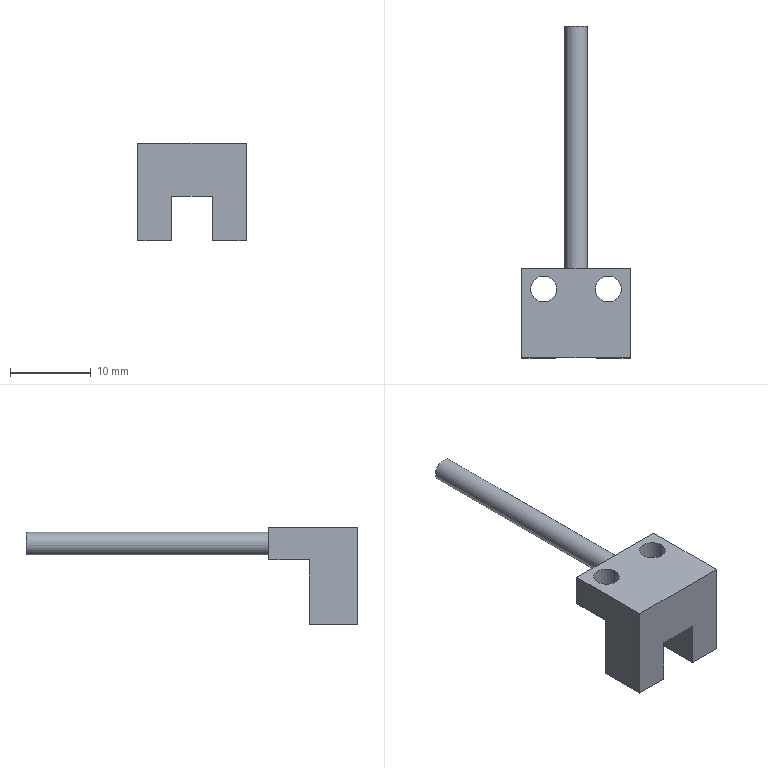Part | STEP file | 1 solid | 16 faces | box 13.4 x 41 x 12 mm | volume 1188 mm3 | plane 13 | cylinder 3 | commonest cylinder face diameters 3.2 x2 2.8 x1
STEP:
#1=CARTESIAN_POINT('',(0.,0.,0.));
#2=DIRECTION('',(0.,0.,1.));
#3=DIRECTION('',(1.,0.,0.));
#4=AXIS2_PLACEMENT_3D('',#1,#2,#3);
#5=CARTESIAN_POINT('',(2.5,0.,-0.5));
#6=VERTEX_POINT('',#5);
#7=CARTESIAN_POINT('',(2.5,0.,-6.));
#8=VERTEX_POINT('',#7);
#9=CARTESIAN_POINT('',(2.5,0.,0.));
#10=DIRECTION('',(0.,0.,-1.));
#11=VECTOR('',#10,1.);
#12=LINE('',#9,#11);
#13=CARTESIAN_POINT('',(0.,0.,0.));
#14=DIRECTION('',(0.,-1.,0.));
#15=DIRECTION('',(0.,0.,-1.));
#16=AXIS2_PLACEMENT_3D('',#13,#14,#15);
#17=PLANE('',#16);
#18=CARTESIAN_POINT('',(0.,2.5));
#19=DIRECTION('',(1.,0.));
#20=VECTOR('',#19,1.);
#21=LINE('',#18,#20);
#22=(GEOMETRIC_REPRESENTATION_CONTEXT(2)PARAMETRIC_REPRESENTATION_CONTEXT()REPRESENTATION_CONTEXT('',''));
#23=DEFINITIONAL_REPRESENTATION('',(#21),#22);
#24=PCURVE('',#17,#23);
#25=CARTESIAN_POINT('',(2.5,11.,-6.));
#26=DIRECTION('',(1.,0.,0.));
#27=DIRECTION('',(0.,0.,-1.));
#28=AXIS2_PLACEMENT_3D('',#25,#26,#27);
#29=PLANE('',#28);
#30=CARTESIAN_POINT('',(-6.,-11.));
#31=DIRECTION('',(1.,0.));
#32=VECTOR('',#31,1.);
#33=LINE('',#30,#32);
#34=(GEOMETRIC_REPRESENTATION_CONTEXT(2)PARAMETRIC_REPRESENTATION_CONTEXT()REPRESENTATION_CONTEXT('',''));
#35=DEFINITIONAL_REPRESENTATION('',(#33),#34);
#36=PCURVE('',#29,#35);
#37=SURFACE_CURVE('',#12,(#24,#36),.PCURVE_S1.);
#38=EDGE_CURVE('',#6,#8,#37,.T.);
#39=ORIENTED_EDGE('',*,*,#38,.T.);
#40=CARTESIAN_POINT('',(6.7,0.,-6.));
#41=VERTEX_POINT('',#40);
#42=CARTESIAN_POINT('',(0.,0.,-6.));
#43=DIRECTION('',(1.,0.,0.));
#44=VECTOR('',#43,1.);
#45=LINE('',#42,#44);
#46=CARTESIAN_POINT('',(6.,0.));
#47=DIRECTION('',(0.,1.));
#48=VECTOR('',#47,1.);
#49=LINE('',#46,#48);
#50=(GEOMETRIC_REPRESENTATION_CONTEXT(2)PARAMETRIC_REPRESENTATION_CONTEXT()REPRESENTATION_CONTEXT('',''));
#51=DEFINITIONAL_REPRESENTATION('',(#49),#50);
#52=PCURVE('',#17,#51);
#53=CARTESIAN_POINT('',(2.5,11.,-6.));
#54=DIRECTION('',(0.,0.,1.));
#55=DIRECTION('',(1.,0.,0.));
#56=AXIS2_PLACEMENT_3D('',#53,#54,#55);
#57=PLANE('',#56);
#58=CARTESIAN_POINT('',(-2.5,-11.));
#59=DIRECTION('',(1.,0.));
#60=VECTOR('',#59,1.);
#61=LINE('',#58,#60);
#62=(GEOMETRIC_REPRESENTATION_CONTEXT(2)PARAMETRIC_REPRESENTATION_CONTEXT()REPRESENTATION_CONTEXT('',''));
#63=DEFINITIONAL_REPRESENTATION('',(#61),#62);
#64=PCURVE('',#57,#63);
#65=SURFACE_CURVE('',#45,(#52,#64),.PCURVE_S1.);
#66=EDGE_CURVE('',#8,#41,#65,.T.);
#67=ORIENTED_EDGE('',*,*,#66,.T.);
#68=CARTESIAN_POINT('',(6.7,0.,6.));
#69=VERTEX_POINT('',#68);
#70=CARTESIAN_POINT('',(6.7,0.,0.));
#71=DIRECTION('',(0.,0.,1.));
#72=VECTOR('',#71,1.);
#73=LINE('',#70,#72);
#74=CARTESIAN_POINT('',(0.,6.7));
#75=DIRECTION('',(-1.,0.));
#76=VECTOR('',#75,1.);
#77=LINE('',#74,#76);
#78=(GEOMETRIC_REPRESENTATION_CONTEXT(2)PARAMETRIC_REPRESENTATION_CONTEXT()REPRESENTATION_CONTEXT('',''));
#79=DEFINITIONAL_REPRESENTATION('',(#77),#78);
#80=PCURVE('',#17,#79);
#81=CARTESIAN_POINT('',(6.7,11.,6.));
#82=DIRECTION('',(-1.,0.,0.));
#83=DIRECTION('',(0.,0.,1.));
#84=AXIS2_PLACEMENT_3D('',#81,#82,#83);
#85=PLANE('',#84);
#86=CARTESIAN_POINT('',(-6.,-11.));
#87=DIRECTION('',(1.,0.));
#88=VECTOR('',#87,1.);
#89=LINE('',#86,#88);
#90=(GEOMETRIC_REPRESENTATION_CONTEXT(2)PARAMETRIC_REPRESENTATION_CONTEXT()REPRESENTATION_CONTEXT('',''));
#91=DEFINITIONAL_REPRESENTATION('',(#89),#90);
#92=PCURVE('',#85,#91);
#93=SURFACE_CURVE('',#73,(#80,#92),.PCURVE_S1.);
#94=EDGE_CURVE('',#41,#69,#93,.T.);
#95=ORIENTED_EDGE('',*,*,#94,.T.);
#96=CARTESIAN_POINT('',(-6.7,0.,6.));
#97=VERTEX_POINT('',#96);
#98=CARTESIAN_POINT('',(0.,0.,6.));
#99=DIRECTION('',(-1.,0.,0.));
#100=VECTOR('',#99,1.);
#101=LINE('',#98,#100);
#102=CARTESIAN_POINT('',(-6.,0.));
#103=DIRECTION('',(0.,-1.));
#104=VECTOR('',#103,1.);
#105=LINE('',#102,#104);
#106=(GEOMETRIC_REPRESENTATION_CONTEXT(2)PARAMETRIC_REPRESENTATION_CONTEXT()REPRESENTATION_CONTEXT('',''));
#107=DEFINITIONAL_REPRESENTATION('',(#105),#106);
#108=PCURVE('',#17,#107);
#109=CARTESIAN_POINT('',(-6.7,11.,6.));
#110=DIRECTION('',(0.,0.,-1.));
#111=DIRECTION('',(-1.,0.,0.));
#112=AXIS2_PLACEMENT_3D('',#109,#110,#111);
#113=PLANE('',#112);
#114=CARTESIAN_POINT('',(-6.7,-11.));
#115=DIRECTION('',(1.,0.));
#116=VECTOR('',#115,1.);
#117=LINE('',#114,#116);
#118=(GEOMETRIC_REPRESENTATION_CONTEXT(2)PARAMETRIC_REPRESENTATION_CONTEXT()REPRESENTATION_CONTEXT('',''));
#119=DEFINITIONAL_REPRESENTATION('',(#117),#118);
#120=PCURVE('',#113,#119);
#121=SURFACE_CURVE('',#101,(#108,#120),.PCURVE_S1.);
#122=EDGE_CURVE('',#69,#97,#121,.T.);
#123=ORIENTED_EDGE('',*,*,#122,.T.);
#124=CARTESIAN_POINT('',(-6.7,0.,-6.));
#125=VERTEX_POINT('',#124);
#126=CARTESIAN_POINT('',(-6.7,0.,0.));
#127=DIRECTION('',(0.,0.,-1.));
#128=VECTOR('',#127,1.);
#129=LINE('',#126,#128);
#130=CARTESIAN_POINT('',(0.,-6.7));
#131=DIRECTION('',(1.,0.));
#132=VECTOR('',#131,1.);
#133=LINE('',#130,#132);
#134=(GEOMETRIC_REPRESENTATION_CONTEXT(2)PARAMETRIC_REPRESENTATION_CONTEXT()REPRESENTATION_CONTEXT('',''));
#135=DEFINITIONAL_REPRESENTATION('',(#133),#134);
#136=PCURVE('',#17,#135);
#137=CARTESIAN_POINT('',(-6.7,11.,6.));
#138=DIRECTION('',(1.,0.,0.));
#139=DIRECTION('',(0.,0.,-1.));
#140=AXIS2_PLACEMENT_3D('',#137,#138,#139);
#141=PLANE('',#140);
#142=CARTESIAN_POINT('',(6.,-11.));
#143=DIRECTION('',(1.,0.));
#144=VECTOR('',#143,1.);
#145=LINE('',#142,#144);
#146=(GEOMETRIC_REPRESENTATION_CONTEXT(2)PARAMETRIC_REPRESENTATION_CONTEXT()REPRESENTATION_CONTEXT('',''));
#147=DEFINITIONAL_REPRESENTATION('',(#145),#146);
#148=PCURVE('',#141,#147);
#149=SURFACE_CURVE('',#129,(#136,#148),.PCURVE_S1.);
#150=EDGE_CURVE('',#97,#125,#149,.T.);
#151=ORIENTED_EDGE('',*,*,#150,.T.);
#152=CARTESIAN_POINT('',(-2.5,0.,-6.));
#153=VERTEX_POINT('',#152);
#154=CARTESIAN_POINT('',(0.,0.,-6.));
#155=DIRECTION('',(1.,0.,0.));
#156=VECTOR('',#155,1.);
#157=LINE('',#154,#156);
#158=CARTESIAN_POINT('',(6.,0.));
#159=DIRECTION('',(0.,1.));
#160=VECTOR('',#159,1.);
#161=LINE('',#158,#160);
#162=(GEOMETRIC_REPRESENTATION_CONTEXT(2)PARAMETRIC_REPRESENTATION_CONTEXT()REPRESENTATION_CONTEXT('',''));
#163=DEFINITIONAL_REPRESENTATION('',(#161),#162);
#164=PCURVE('',#17,#163);
#165=CARTESIAN_POINT('',(-6.7,11.,-6.));
#166=DIRECTION('',(0.,0.,1.));
#167=DIRECTION('',(1.,0.,0.));
#168=AXIS2_PLACEMENT_3D('',#165,#166,#167);
#169=PLANE('',#168);
#170=CARTESIAN_POINT('',(6.7,-11.));
#171=DIRECTION('',(1.,0.));
#172=VECTOR('',#171,1.);
#173=LINE('',#170,#172);
#174=(GEOMETRIC_REPRESENTATION_CONTEXT(2)PARAMETRIC_REPRESENTATION_CONTEXT()REPRESENTATION_CONTEXT('',''));
#175=DEFINITIONAL_REPRESENTATION('',(#173),#174);
#176=PCURVE('',#169,#175);
#177=SURFACE_CURVE('',#157,(#164,#176),.PCURVE_S1.);
#178=EDGE_CURVE('',#125,#153,#177,.T.);
#179=ORIENTED_EDGE('',*,*,#178,.T.);
#180=CARTESIAN_POINT('',(-2.5,0.,-0.5));
#181=VERTEX_POINT('',#180);
#182=CARTESIAN_POINT('',(-2.5,0.,0.));
#183=DIRECTION('',(0.,0.,1.));
#184=VECTOR('',#183,1.);
#185=LINE('',#182,#184);
#186=CARTESIAN_POINT('',(0.,-2.5));
#187=DIRECTION('',(-1.,0.));
#188=VECTOR('',#187,1.);
#189=LINE('',#186,#188);
#190=(GEOMETRIC_REPRESENTATION_CONTEXT(2)PARAMETRIC_REPRESENTATION_CONTEXT()REPRESENTATION_CONTEXT('',''));
#191=DEFINITIONAL_REPRESENTATION('',(#189),#190);
#192=PCURVE('',#17,#191);
#193=CARTESIAN_POINT('',(-2.5,11.,-6.));
#194=DIRECTION('',(-1.,0.,0.));
#195=DIRECTION('',(0.,0.,1.));
#196=AXIS2_PLACEMENT_3D('',#193,#194,#195);
#197=PLANE('',#196);
#198=CARTESIAN_POINT('',(6.,-11.));
#199=DIRECTION('',(1.,0.));
#200=VECTOR('',#199,1.);
#201=LINE('',#198,#200);
#202=(GEOMETRIC_REPRESENTATION_CONTEXT(2)PARAMETRIC_REPRESENTATION_CONTEXT()REPRESENTATION_CONTEXT('',''));
#203=DEFINITIONAL_REPRESENTATION('',(#201),#202);
#204=PCURVE('',#197,#203);
#205=SURFACE_CURVE('',#185,(#192,#204),.PCURVE_S1.);
#206=EDGE_CURVE('',#153,#181,#205,.T.);
#207=ORIENTED_EDGE('',*,*,#206,.T.);
#208=CARTESIAN_POINT('',(0.,0.,-0.5));
#209=DIRECTION('',(1.,0.,0.));
#210=VECTOR('',#209,1.);
#211=LINE('',#208,#210);
#212=CARTESIAN_POINT('',(0.5,0.));
#213=DIRECTION('',(0.,1.));
#214=VECTOR('',#213,1.);
#215=LINE('',#212,#214);
#216=(GEOMETRIC_REPRESENTATION_CONTEXT(2)PARAMETRIC_REPRESENTATION_CONTEXT()REPRESENTATION_CONTEXT('',''));
#217=DEFINITIONAL_REPRESENTATION('',(#215),#216);
#218=PCURVE('',#17,#217);
#219=CARTESIAN_POINT('',(-2.5,11.,-0.5));
#220=DIRECTION('',(0.,0.,1.));
#221=DIRECTION('',(0.,-1.,0.));
#222=AXIS2_PLACEMENT_3D('',#219,#220,#221);
#223=PLANE('',#222);
#224=CARTESIAN_POINT('',(11.,2.5));
#225=DIRECTION('',(0.,1.));
#226=VECTOR('',#225,1.);
#227=LINE('',#224,#226);
#228=(GEOMETRIC_REPRESENTATION_CONTEXT(2)PARAMETRIC_REPRESENTATION_CONTEXT()REPRESENTATION_CONTEXT('',''));
#229=DEFINITIONAL_REPRESENTATION('',(#227),#228);
#230=PCURVE('',#223,#229);
#231=SURFACE_CURVE('',#211,(#218,#230),.PCURVE_S1.);
#232=EDGE_CURVE('',#181,#6,#231,.T.);
#233=ORIENTED_EDGE('',*,*,#232,.T.);
#234=EDGE_LOOP('',(#39,#67,#95,#123,#151,#179,#207,#233));
#235=FACE_BOUND('',#234,.T.);
#236=ADVANCED_FACE('',(#235),#17,.T.);
#237=CARTESIAN_POINT('',(6.7,6.,-6.));
#238=VERTEX_POINT('',#237);
#239=CARTESIAN_POINT('',(6.7,11.,-6.));
#240=DIRECTION('',(0.,1.,0.));
#241=VECTOR('',#240,1.);
#242=LINE('',#239,#241);
#243=CARTESIAN_POINT('',(4.2,0.));
#244=DIRECTION('',(0.,1.));
#245=VECTOR('',#244,1.);
#246=LINE('',#243,#245);
#247=(GEOMETRIC_REPRESENTATION_CONTEXT(2)PARAMETRIC_REPRESENTATION_CONTEXT()REPRESENTATION_CONTEXT('',''));
#248=DEFINITIONAL_REPRESENTATION('',(#246),#247);
#249=PCURVE('',#57,#248);
#250=CARTESIAN_POINT('',(-12.,0.));
#251=DIRECTION('',(0.,1.));
#252=VECTOR('',#251,1.);
#253=LINE('',#250,#252);
#254=(GEOMETRIC_REPRESENTATION_CONTEXT(2)PARAMETRIC_REPRESENTATION_CONTEXT()REPRESENTATION_CONTEXT('',''));
#255=DEFINITIONAL_REPRESENTATION('',(#253),#254);
#256=PCURVE('',#85,#255);
#257=SURFACE_CURVE('',#242,(#249,#256),.PCURVE_S1.);
#258=EDGE_CURVE('',#41,#238,#257,.T.);
#259=ORIENTED_EDGE('',*,*,#258,.F.);
#260=ORIENTED_EDGE('',*,*,#66,.F.);
#261=CARTESIAN_POINT('',(2.5,6.,-6.));
#262=VERTEX_POINT('',#261);
#263=CARTESIAN_POINT('',(2.5,11.,-6.));
#264=DIRECTION('',(0.,-1.,0.));
#265=VECTOR('',#264,1.);
#266=LINE('',#263,#265);
#267=CARTESIAN_POINT('',(0.,0.));
#268=DIRECTION('',(0.,-1.));
#269=VECTOR('',#268,1.);
#270=LINE('',#267,#269);
#271=(GEOMETRIC_REPRESENTATION_CONTEXT(2)PARAMETRIC_REPRESENTATION_CONTEXT()REPRESENTATION_CONTEXT('',''));
#272=DEFINITIONAL_REPRESENTATION('',(#270),#271);
#273=PCURVE('',#57,#272);
#274=CARTESIAN_POINT('',(0.,0.));
#275=DIRECTION('',(0.,-1.));
#276=VECTOR('',#275,1.);
#277=LINE('',#274,#276);
#278=(GEOMETRIC_REPRESENTATION_CONTEXT(2)PARAMETRIC_REPRESENTATION_CONTEXT()REPRESENTATION_CONTEXT('',''));
#279=DEFINITIONAL_REPRESENTATION('',(#277),#278);
#280=PCURVE('',#29,#279);
#281=SURFACE_CURVE('',#266,(#273,#280),.PCURVE_S1.);
#282=EDGE_CURVE('',#262,#8,#281,.T.);
#283=ORIENTED_EDGE('',*,*,#282,.F.);
#284=CARTESIAN_POINT('',(2.5,6.,-6.));
#285=DIRECTION('',(-1.,0.,0.));
#286=VECTOR('',#285,1.);
#287=LINE('',#284,#286);
#288=CARTESIAN_POINT('',(0.,-5.));
#289=DIRECTION('',(-1.,0.));
#290=VECTOR('',#289,1.);
#291=LINE('',#288,#290);
#292=(GEOMETRIC_REPRESENTATION_CONTEXT(2)PARAMETRIC_REPRESENTATION_CONTEXT()REPRESENTATION_CONTEXT('',''));
#293=DEFINITIONAL_REPRESENTATION('',(#291),#292);
#294=PCURVE('',#57,#293);
#295=CARTESIAN_POINT('',(0.,6.,0.));
#296=DIRECTION('',(0.,1.,0.));
#297=DIRECTION('',(0.,0.,1.));
#298=AXIS2_PLACEMENT_3D('',#295,#296,#297);
#299=PLANE('',#298);
#300=CARTESIAN_POINT('',(-6.,2.5));
#301=DIRECTION('',(0.,-1.));
#302=VECTOR('',#301,1.);
#303=LINE('',#300,#302);
#304=(GEOMETRIC_REPRESENTATION_CONTEXT(2)PARAMETRIC_REPRESENTATION_CONTEXT()REPRESENTATION_CONTEXT('',''));
#305=DEFINITIONAL_REPRESENTATION('',(#303),#304);
#306=PCURVE('',#299,#305);
#307=SURFACE_CURVE('',#287,(#294,#306),.PCURVE_S1.);
#308=EDGE_CURVE('',#238,#262,#307,.T.);
#309=ORIENTED_EDGE('',*,*,#308,.F.);
#310=EDGE_LOOP('',(#259,#260,#283,#309));
#311=FACE_BOUND('',#310,.T.);
#312=ADVANCED_FACE('',(#311),#57,.F.);
#313=ORIENTED_EDGE('',*,*,#282,.T.);
#314=ORIENTED_EDGE('',*,*,#38,.F.);
#315=CARTESIAN_POINT('',(2.5,6.,-0.5));
#316=VERTEX_POINT('',#315);
#317=CARTESIAN_POINT('',(2.5,11.,-0.5));
#318=DIRECTION('',(0.,-1.,0.));
#319=VECTOR('',#318,1.);
#320=LINE('',#317,#319);
#321=CARTESIAN_POINT('',(-5.5,0.));
#322=DIRECTION('',(0.,-1.));
#323=VECTOR('',#322,1.);
#324=LINE('',#321,#323);
#325=(GEOMETRIC_REPRESENTATION_CONTEXT(2)PARAMETRIC_REPRESENTATION_CONTEXT()REPRESENTATION_CONTEXT('',''));
#326=DEFINITIONAL_REPRESENTATION('',(#324),#325);
#327=PCURVE('',#29,#326);
#328=CARTESIAN_POINT('',(0.,5.));
#329=DIRECTION('',(1.,0.));
#330=VECTOR('',#329,1.);
#331=LINE('',#328,#330);
#332=(GEOMETRIC_REPRESENTATION_CONTEXT(2)PARAMETRIC_REPRESENTATION_CONTEXT()REPRESENTATION_CONTEXT('',''));
#333=DEFINITIONAL_REPRESENTATION('',(#331),#332);
#334=PCURVE('',#223,#333);
#335=SURFACE_CURVE('',#320,(#327,#334),.PCURVE_S1.);
#336=EDGE_CURVE('',#316,#6,#335,.T.);
#337=ORIENTED_EDGE('',*,*,#336,.F.);
#338=CARTESIAN_POINT('',(2.5,6.,-6.));
#339=DIRECTION('',(0.,0.,1.));
#340=VECTOR('',#339,1.);
#341=LINE('',#338,#340);
#342=CARTESIAN_POINT('',(0.,-5.));
#343=DIRECTION('',(-1.,0.));
#344=VECTOR('',#343,1.);
#345=LINE('',#342,#344);
#346=(GEOMETRIC_REPRESENTATION_CONTEXT(2)PARAMETRIC_REPRESENTATION_CONTEXT()REPRESENTATION_CONTEXT('',''));
#347=DEFINITIONAL_REPRESENTATION('',(#345),#346);
#348=PCURVE('',#29,#347);
#349=CARTESIAN_POINT('',(-6.,2.5));
#350=DIRECTION('',(1.,0.));
#351=VECTOR('',#350,1.);
#352=LINE('',#349,#351);
#353=(GEOMETRIC_REPRESENTATION_CONTEXT(2)PARAMETRIC_REPRESENTATION_CONTEXT()REPRESENTATION_CONTEXT('',''));
#354=DEFINITIONAL_REPRESENTATION('',(#352),#353);
#355=PCURVE('',#299,#354);
#356=SURFACE_CURVE('',#341,(#348,#355),.PCURVE_S1.);
#357=EDGE_CURVE('',#262,#316,#356,.T.);
#358=ORIENTED_EDGE('',*,*,#357,.F.);
#359=EDGE_LOOP('',(#313,#314,#337,#358));
#360=FACE_BOUND('',#359,.T.);
#361=ADVANCED_FACE('',(#360),#29,.F.);
#362=ORIENTED_EDGE('',*,*,#336,.T.);
#363=ORIENTED_EDGE('',*,*,#232,.F.);
#364=CARTESIAN_POINT('',(-2.5,6.,-0.5));
#365=VERTEX_POINT('',#364);
#366=CARTESIAN_POINT('',(-2.5,11.,-0.5));
#367=DIRECTION('',(0.,-1.,0.));
#368=VECTOR('',#367,1.);
#369=LINE('',#366,#368);
#370=CARTESIAN_POINT('',(0.,0.));
#371=DIRECTION('',(1.,0.));
#372=VECTOR('',#371,1.);
#373=LINE('',#370,#372);
#374=(GEOMETRIC_REPRESENTATION_CONTEXT(2)PARAMETRIC_REPRESENTATION_CONTEXT()REPRESENTATION_CONTEXT('',''));
#375=DEFINITIONAL_REPRESENTATION('',(#373),#374);
#376=PCURVE('',#223,#375);
#377=CARTESIAN_POINT('',(5.5,0.));
#378=DIRECTION('',(0.,-1.));
#379=VECTOR('',#378,1.);
#380=LINE('',#377,#379);
#381=(GEOMETRIC_REPRESENTATION_CONTEXT(2)PARAMETRIC_REPRESENTATION_CONTEXT()REPRESENTATION_CONTEXT('',''));
#382=DEFINITIONAL_REPRESENTATION('',(#380),#381);
#383=PCURVE('',#197,#382);
#384=SURFACE_CURVE('',#369,(#376,#383),.PCURVE_S1.);
#385=EDGE_CURVE('',#365,#181,#384,.T.);
#386=ORIENTED_EDGE('',*,*,#385,.F.);
#387=CARTESIAN_POINT('',(-2.5,6.,-0.5));
#388=DIRECTION('',(-1.,0.,0.));
#389=VECTOR('',#388,1.);
#390=LINE('',#387,#389);
#391=CARTESIAN_POINT('',(5.,0.));
#392=DIRECTION('',(0.,-1.));
#393=VECTOR('',#392,1.);
#394=LINE('',#391,#393);
#395=(GEOMETRIC_REPRESENTATION_CONTEXT(2)PARAMETRIC_REPRESENTATION_CONTEXT()REPRESENTATION_CONTEXT('',''));
#396=DEFINITIONAL_REPRESENTATION('',(#394),#395);
#397=PCURVE('',#223,#396);
#398=CARTESIAN_POINT('',(-0.5,-2.5));
#399=DIRECTION('',(0.,-1.));
#400=VECTOR('',#399,1.);
#401=LINE('',#398,#400);
#402=(GEOMETRIC_REPRESENTATION_CONTEXT(2)PARAMETRIC_REPRESENTATION_CONTEXT()REPRESENTATION_CONTEXT('',''));
#403=DEFINITIONAL_REPRESENTATION('',(#401),#402);
#404=PCURVE('',#299,#403);
#405=SURFACE_CURVE('',#390,(#397,#404),.PCURVE_S1.);
#406=EDGE_CURVE('',#316,#365,#405,.T.);
#407=ORIENTED_EDGE('',*,*,#406,.F.);
#408=EDGE_LOOP('',(#362,#363,#386,#407));
#409=FACE_BOUND('',#408,.T.);
#410=ADVANCED_FACE('',(#409),#223,.F.);
#411=ORIENTED_EDGE('',*,*,#385,.T.);
#412=ORIENTED_EDGE('',*,*,#206,.F.);
#413=CARTESIAN_POINT('',(-2.5,6.,-6.));
#414=VERTEX_POINT('',#413);
#415=CARTESIAN_POINT('',(-2.5,11.,-6.));
#416=DIRECTION('',(0.,-1.,0.));
#417=VECTOR('',#416,1.);
#418=LINE('',#415,#417);
#419=CARTESIAN_POINT('',(0.,0.));
#420=DIRECTION('',(0.,-1.));
#421=VECTOR('',#420,1.);
#422=LINE('',#419,#421);
#423=(GEOMETRIC_REPRESENTATION_CONTEXT(2)PARAMETRIC_REPRESENTATION_CONTEXT()REPRESENTATION_CONTEXT('',''));
#424=DEFINITIONAL_REPRESENTATION('',(#422),#423);
#425=PCURVE('',#197,#424);
#426=CARTESIAN_POINT('',(4.2,0.));
#427=DIRECTION('',(0.,-1.));
#428=VECTOR('',#427,1.);
#429=LINE('',#426,#428);
#430=(GEOMETRIC_REPRESENTATION_CONTEXT(2)PARAMETRIC_REPRESENTATION_CONTEXT()REPRESENTATION_CONTEXT('',''));
#431=DEFINITIONAL_REPRESENTATION('',(#429),#430);
#432=PCURVE('',#169,#431);
#433=SURFACE_CURVE('',#418,(#425,#432),.PCURVE_S1.);
#434=EDGE_CURVE('',#414,#153,#433,.T.);
#435=ORIENTED_EDGE('',*,*,#434,.F.);
#436=CARTESIAN_POINT('',(-2.5,6.,-6.));
#437=DIRECTION('',(0.,0.,-1.));
#438=VECTOR('',#437,1.);
#439=LINE('',#436,#438);
#440=CARTESIAN_POINT('',(0.,-5.));
#441=DIRECTION('',(-1.,0.));
#442=VECTOR('',#441,1.);
#443=LINE('',#440,#442);
#444=(GEOMETRIC_REPRESENTATION_CONTEXT(2)PARAMETRIC_REPRESENTATION_CONTEXT()REPRESENTATION_CONTEXT('',''));
#445=DEFINITIONAL_REPRESENTATION('',(#443),#444);
#446=PCURVE('',#197,#445);
#447=CARTESIAN_POINT('',(-6.,-2.5));
#448=DIRECTION('',(-1.,0.));
#449=VECTOR('',#448,1.);
#450=LINE('',#447,#449);
#451=(GEOMETRIC_REPRESENTATION_CONTEXT(2)PARAMETRIC_REPRESENTATION_CONTEXT()REPRESENTATION_CONTEXT('',''));
#452=DEFINITIONAL_REPRESENTATION('',(#450),#451);
#453=PCURVE('',#299,#452);
#454=SURFACE_CURVE('',#439,(#446,#453),.PCURVE_S1.);
#455=EDGE_CURVE('',#365,#414,#454,.T.);
#456=ORIENTED_EDGE('',*,*,#455,.F.);
#457=EDGE_LOOP('',(#411,#412,#435,#456));
#458=FACE_BOUND('',#457,.T.);
#459=ADVANCED_FACE('',(#458),#197,.F.);
#460=ORIENTED_EDGE('',*,*,#434,.T.);
#461=ORIENTED_EDGE('',*,*,#178,.F.);
#462=CARTESIAN_POINT('',(-6.7,6.,-6.));
#463=VERTEX_POINT('',#462);
#464=CARTESIAN_POINT('',(-6.7,11.,-6.));
#465=DIRECTION('',(0.,-1.,0.));
#466=VECTOR('',#465,1.);
#467=LINE('',#464,#466);
#468=CARTESIAN_POINT('',(0.,0.));
#469=DIRECTION('',(0.,-1.));
#470=VECTOR('',#469,1.);
#471=LINE('',#468,#470);
#472=(GEOMETRIC_REPRESENTATION_CONTEXT(2)PARAMETRIC_REPRESENTATION_CONTEXT()REPRESENTATION_CONTEXT('',''));
#473=DEFINITIONAL_REPRESENTATION('',(#471),#472);
#474=PCURVE('',#169,#473);
#475=CARTESIAN_POINT('',(12.,0.));
#476=DIRECTION('',(0.,-1.));
#477=VECTOR('',#476,1.);
#478=LINE('',#475,#477);
#479=(GEOMETRIC_REPRESENTATION_CONTEXT(2)PARAMETRIC_REPRESENTATION_CONTEXT()REPRESENTATION_CONTEXT('',''));
#480=DEFINITIONAL_REPRESENTATION('',(#478),#479);
#481=PCURVE('',#141,#480);
#482=SURFACE_CURVE('',#467,(#474,#481),.PCURVE_S1.);
#483=EDGE_CURVE('',#463,#125,#482,.T.);
#484=ORIENTED_EDGE('',*,*,#483,.F.);
#485=CARTESIAN_POINT('',(-6.7,6.,-6.));
#486=DIRECTION('',(-1.,0.,0.));
#487=VECTOR('',#486,1.);
#488=LINE('',#485,#487);
#489=CARTESIAN_POINT('',(0.,-5.));
#490=DIRECTION('',(-1.,0.));
#491=VECTOR('',#490,1.);
#492=LINE('',#489,#491);
#493=(GEOMETRIC_REPRESENTATION_CONTEXT(2)PARAMETRIC_REPRESENTATION_CONTEXT()REPRESENTATION_CONTEXT('',''));
#494=DEFINITIONAL_REPRESENTATION('',(#492),#493);
#495=PCURVE('',#169,#494);
#496=CARTESIAN_POINT('',(-6.,-6.7));
#497=DIRECTION('',(0.,-1.));
#498=VECTOR('',#497,1.);
#499=LINE('',#496,#498);
#500=(GEOMETRIC_REPRESENTATION_CONTEXT(2)PARAMETRIC_REPRESENTATION_CONTEXT()REPRESENTATION_CONTEXT('',''));
#501=DEFINITIONAL_REPRESENTATION('',(#499),#500);
#502=PCURVE('',#299,#501);
#503=SURFACE_CURVE('',#488,(#495,#502),.PCURVE_S1.);
#504=EDGE_CURVE('',#414,#463,#503,.T.);
#505=ORIENTED_EDGE('',*,*,#504,.F.);
#506=EDGE_LOOP('',(#460,#461,#484,#505));
#507=FACE_BOUND('',#506,.T.);
#508=ADVANCED_FACE('',(#507),#169,.F.);
#509=CARTESIAN_POINT('',(-6.7,6.,2.));
#510=VERTEX_POINT('',#509);
#511=CARTESIAN_POINT('',(-6.7,11.,2.));
#512=VERTEX_POINT('',#511);
#513=CARTESIAN_POINT('',(-6.7,11.,2.));
#514=DIRECTION('',(0.,1.,0.));
#515=VECTOR('',#514,1.);
#516=LINE('',#513,#515);
#517=CARTESIAN_POINT('',(4.,0.));
#518=DIRECTION('',(0.,1.));
#519=VECTOR('',#518,1.);
#520=LINE('',#517,#519);
#521=(GEOMETRIC_REPRESENTATION_CONTEXT(2)PARAMETRIC_REPRESENTATION_CONTEXT()REPRESENTATION_CONTEXT('',''));
#522=DEFINITIONAL_REPRESENTATION('',(#520),#521);
#523=PCURVE('',#141,#522);
#524=CARTESIAN_POINT('',(-9.583,6.,2.));
#525=DIRECTION('',(0.,0.,1.));
#526=DIRECTION('',(1.,0.,0.));
#527=AXIS2_PLACEMENT_3D('',#524,#525,#526);
#528=PLANE('',#527);
#529=CARTESIAN_POINT('',(2.883,5.));
#530=DIRECTION('',(0.,1.));
#531=VECTOR('',#530,1.);
#532=LINE('',#529,#531);
#533=(GEOMETRIC_REPRESENTATION_CONTEXT(2)PARAMETRIC_REPRESENTATION_CONTEXT()REPRESENTATION_CONTEXT('',''));
#534=DEFINITIONAL_REPRESENTATION('',(#532),#533);
#535=PCURVE('',#528,#534);
#536=SURFACE_CURVE('',#516,(#523,#535),.PCURVE_S1.);
#537=EDGE_CURVE('',#510,#512,#536,.T.);
#538=ORIENTED_EDGE('',*,*,#537,.F.);
#539=CARTESIAN_POINT('',(-6.7,6.,6.));
#540=DIRECTION('',(0.,0.,1.));
#541=VECTOR('',#540,1.);
#542=LINE('',#539,#541);
#543=CARTESIAN_POINT('',(0.,-5.));
#544=DIRECTION('',(-1.,0.));
#545=VECTOR('',#544,1.);
#546=LINE('',#543,#545);
#547=(GEOMETRIC_REPRESENTATION_CONTEXT(2)PARAMETRIC_REPRESENTATION_CONTEXT()REPRESENTATION_CONTEXT('',''));
#548=DEFINITIONAL_REPRESENTATION('',(#546),#547);
#549=PCURVE('',#141,#548);
#550=CARTESIAN_POINT('',(6.,-6.7));
#551=DIRECTION('',(1.,0.));
#552=VECTOR('',#551,1.);
#553=LINE('',#550,#552);
#554=(GEOMETRIC_REPRESENTATION_CONTEXT(2)PARAMETRIC_REPRESENTATION_CONTEXT()REPRESENTATION_CONTEXT('',''));
#555=DEFINITIONAL_REPRESENTATION('',(#553),#554);
#556=PCURVE('',#299,#555);
#557=SURFACE_CURVE('',#542,(#549,#556),.PCURVE_S1.);
#558=EDGE_CURVE('',#463,#510,#557,.T.);
#559=ORIENTED_EDGE('',*,*,#558,.F.);
#560=ORIENTED_EDGE('',*,*,#483,.T.);
#561=ORIENTED_EDGE('',*,*,#150,.F.);
#562=CARTESIAN_POINT('',(-6.7,11.,6.));
#563=VERTEX_POINT('',#562);
#564=CARTESIAN_POINT('',(-6.7,11.,6.));
#565=DIRECTION('',(0.,-1.,0.));
#566=VECTOR('',#565,1.);
#567=LINE('',#564,#566);
#568=CARTESIAN_POINT('',(0.,0.));
#569=DIRECTION('',(0.,-1.));
#570=VECTOR('',#569,1.);
#571=LINE('',#568,#570);
#572=(GEOMETRIC_REPRESENTATION_CONTEXT(2)PARAMETRIC_REPRESENTATION_CONTEXT()REPRESENTATION_CONTEXT('',''));
#573=DEFINITIONAL_REPRESENTATION('',(#571),#572);
#574=PCURVE('',#141,#573);
#575=CARTESIAN_POINT('',(0.,0.));
#576=DIRECTION('',(0.,-1.));
#577=VECTOR('',#576,1.);
#578=LINE('',#575,#577);
#579=(GEOMETRIC_REPRESENTATION_CONTEXT(2)PARAMETRIC_REPRESENTATION_CONTEXT()REPRESENTATION_CONTEXT('',''));
#580=DEFINITIONAL_REPRESENTATION('',(#578),#579);
#581=PCURVE('',#113,#580);
#582=SURFACE_CURVE('',#567,(#574,#581),.PCURVE_S1.);
#583=EDGE_CURVE('',#563,#97,#582,.T.);
#584=ORIENTED_EDGE('',*,*,#583,.F.);
#585=CARTESIAN_POINT('',(-6.7,11.,6.));
#586=DIRECTION('',(0.,0.,1.));
#587=VECTOR('',#586,1.);
#588=LINE('',#585,#587);
#589=CARTESIAN_POINT('',(0.,0.));
#590=DIRECTION('',(-1.,0.));
#591=VECTOR('',#590,1.);
#592=LINE('',#589,#591);
#593=(GEOMETRIC_REPRESENTATION_CONTEXT(2)PARAMETRIC_REPRESENTATION_CONTEXT()REPRESENTATION_CONTEXT('',''));
#594=DEFINITIONAL_REPRESENTATION('',(#592),#593);
#595=PCURVE('',#141,#594);
#596=CARTESIAN_POINT('',(0.,11.,0.));
#597=DIRECTION('',(0.,-1.,0.));
#598=DIRECTION('',(0.,0.,-1.));
#599=AXIS2_PLACEMENT_3D('',#596,#597,#598);
#600=PLANE('',#599);
#601=CARTESIAN_POINT('',(-6.,-6.7));
#602=DIRECTION('',(-1.,0.));
#603=VECTOR('',#602,1.);
#604=LINE('',#601,#603);
#605=(GEOMETRIC_REPRESENTATION_CONTEXT(2)PARAMETRIC_REPRESENTATION_CONTEXT()REPRESENTATION_CONTEXT('',''));
#606=DEFINITIONAL_REPRESENTATION('',(#604),#605);
#607=PCURVE('',#600,#606);
#608=SURFACE_CURVE('',#588,(#595,#607),.PCURVE_S1.);
#609=EDGE_CURVE('',#512,#563,#608,.T.);
#610=ORIENTED_EDGE('',*,*,#609,.F.);
#611=EDGE_LOOP('',(#538,#559,#560,#561,#584,#610));
#612=FACE_BOUND('',#611,.T.);
#613=ADVANCED_FACE('',(#612),#141,.F.);
#614=CARTESIAN_POINT('',(-5.6,8.5,6.));
#615=VERTEX_POINT('',#614);
#616=CARTESIAN_POINT('',(-4.,8.5,6.));
#617=DIRECTION('',(0.,0.,1.));
#618=DIRECTION('',(-1.,0.,0.));
#619=AXIS2_PLACEMENT_3D('',#616,#617,#618);
#620=CIRCLE('',#619,1.6);
#621=CARTESIAN_POINT('',(-1.1,-2.5));
#622=CARTESIAN_POINT('',(-1.1,-5.271));
#623=CARTESIAN_POINT('',(-3.5,-3.886));
#624=CARTESIAN_POINT('',(-5.9,-2.5));
#625=CARTESIAN_POINT('',(-3.5,-1.114));
#626=CARTESIAN_POINT('',(-1.1,0.2713));
#627=CARTESIAN_POINT('',(-1.1,-2.5));
#628=(BOUNDED_CURVE()B_SPLINE_CURVE(2,(#621,#622,#623,#624,#625,#626,#627),.UNSPECIFIED.,.T.,.F.)B_SPLINE_CURVE_WITH_KNOTS((1,2,2,2,2,1),(-2.094,0.,2.094,4.189,6.283,8.378),.UNSPECIFIED.)CURVE()GEOMETRIC_REPRESENTATION_ITEM()RATIONAL_B_SPLINE_CURVE((1.,0.5,1.,0.5,1.,0.5,1.))REPRESENTATION_ITEM(''));
#629=(GEOMETRIC_REPRESENTATION_CONTEXT(2)PARAMETRIC_REPRESENTATION_CONTEXT()REPRESENTATION_CONTEXT('',''));
#630=DEFINITIONAL_REPRESENTATION('',(#628),#629);
#631=PCURVE('',#113,#630);
#632=CARTESIAN_POINT('',(-4.,8.5,7.));
#633=DIRECTION('',(0.,0.,-1.));
#634=DIRECTION('',(-1.,0.,0.));
#635=AXIS2_PLACEMENT_3D('',#632,#633,#634);
#636=CYLINDRICAL_SURFACE('',#635,1.6);
#637=CARTESIAN_POINT('',(6.283,1.));
#638=DIRECTION('',(-1.,0.));
#639=VECTOR('',#638,1.);
#640=LINE('',#637,#639);
#641=(GEOMETRIC_REPRESENTATION_CONTEXT(2)PARAMETRIC_REPRESENTATION_CONTEXT()REPRESENTATION_CONTEXT('',''));
#642=DEFINITIONAL_REPRESENTATION('',(#640),#641);
#643=PCURVE('',#636,#642);
#644=SURFACE_CURVE('',#620,(#631,#643),.PCURVE_S1.);
#645=EDGE_CURVE('',#615,#615,#644,.T.);
#646=ORIENTED_EDGE('',*,*,#645,.F.);
#647=EDGE_LOOP('',(#646));
#648=FACE_BOUND('',#647,.T.);
#649=CARTESIAN_POINT('',(2.4,8.5,6.));
#650=VERTEX_POINT('',#649);
#651=CARTESIAN_POINT('',(4.,8.5,6.));
#652=DIRECTION('',(0.,0.,1.));
#653=DIRECTION('',(-1.,0.,0.));
#654=AXIS2_PLACEMENT_3D('',#651,#652,#653);
#655=CIRCLE('',#654,1.6);
#656=CARTESIAN_POINT('',(-9.1,-2.5));
#657=CARTESIAN_POINT('',(-9.1,-5.271));
#658=CARTESIAN_POINT('',(-11.5,-3.886));
#659=CARTESIAN_POINT('',(-13.9,-2.5));
#660=CARTESIAN_POINT('',(-11.5,-1.114));
#661=CARTESIAN_POINT('',(-9.1,0.2713));
#662=CARTESIAN_POINT('',(-9.1,-2.5));
#663=(BOUNDED_CURVE()B_SPLINE_CURVE(2,(#656,#657,#658,#659,#660,#661,#662),.UNSPECIFIED.,.T.,.F.)B_SPLINE_CURVE_WITH_KNOTS((1,2,2,2,2,1),(-2.094,0.,2.094,4.189,6.283,8.378),.UNSPECIFIED.)CURVE()GEOMETRIC_REPRESENTATION_ITEM()RATIONAL_B_SPLINE_CURVE((1.,0.5,1.,0.5,1.,0.5,1.))REPRESENTATION_ITEM(''));
#664=(GEOMETRIC_REPRESENTATION_CONTEXT(2)PARAMETRIC_REPRESENTATION_CONTEXT()REPRESENTATION_CONTEXT('',''));
#665=DEFINITIONAL_REPRESENTATION('',(#663),#664);
#666=PCURVE('',#113,#665);
#667=CARTESIAN_POINT('',(4.,8.5,7.));
#668=DIRECTION('',(0.,0.,-1.));
#669=DIRECTION('',(-1.,0.,0.));
#670=AXIS2_PLACEMENT_3D('',#667,#668,#669);
#671=CYLINDRICAL_SURFACE('',#670,1.6);
#672=CARTESIAN_POINT('',(6.283,1.));
#673=DIRECTION('',(-1.,0.));
#674=VECTOR('',#673,1.);
#675=LINE('',#672,#674);
#676=(GEOMETRIC_REPRESENTATION_CONTEXT(2)PARAMETRIC_REPRESENTATION_CONTEXT()REPRESENTATION_CONTEXT('',''));
#677=DEFINITIONAL_REPRESENTATION('',(#675),#676);
#678=PCURVE('',#671,#677);
#679=SURFACE_CURVE('',#655,(#666,#678),.PCURVE_S1.);
#680=EDGE_CURVE('',#650,#650,#679,.T.);
#681=ORIENTED_EDGE('',*,*,#680,.F.);
#682=EDGE_LOOP('',(#681));
#683=FACE_BOUND('',#682,.T.);
#684=CARTESIAN_POINT('',(6.7,11.,6.));
#685=VERTEX_POINT('',#684);
#686=CARTESIAN_POINT('',(6.7,11.,6.));
#687=DIRECTION('',(0.,-1.,0.));
#688=VECTOR('',#687,1.);
#689=LINE('',#686,#688);
#690=CARTESIAN_POINT('',(-13.4,0.));
#691=DIRECTION('',(0.,-1.));
#692=VECTOR('',#691,1.);
#693=LINE('',#690,#692);
#694=(GEOMETRIC_REPRESENTATION_CONTEXT(2)PARAMETRIC_REPRESENTATION_CONTEXT()REPRESENTATION_CONTEXT('',''));
#695=DEFINITIONAL_REPRESENTATION('',(#693),#694);
#696=PCURVE('',#113,#695);
#697=CARTESIAN_POINT('',(0.,0.));
#698=DIRECTION('',(0.,-1.));
#699=VECTOR('',#698,1.);
#700=LINE('',#697,#699);
#701=(GEOMETRIC_REPRESENTATION_CONTEXT(2)PARAMETRIC_REPRESENTATION_CONTEXT()REPRESENTATION_CONTEXT('',''));
#702=DEFINITIONAL_REPRESENTATION('',(#700),#701);
#703=PCURVE('',#85,#702);
#704=SURFACE_CURVE('',#689,(#696,#703),.PCURVE_S1.);
#705=EDGE_CURVE('',#685,#69,#704,.T.);
#706=ORIENTED_EDGE('',*,*,#705,.F.);
#707=CARTESIAN_POINT('',(-6.7,11.,6.));
#708=DIRECTION('',(1.,0.,0.));
#709=VECTOR('',#708,1.);
#710=LINE('',#707,#709);
#711=CARTESIAN_POINT('',(0.,0.));
#712=DIRECTION('',(-1.,0.));
#713=VECTOR('',#712,1.);
#714=LINE('',#711,#713);
#715=(GEOMETRIC_REPRESENTATION_CONTEXT(2)PARAMETRIC_REPRESENTATION_CONTEXT()REPRESENTATION_CONTEXT('',''));
#716=DEFINITIONAL_REPRESENTATION('',(#714),#715);
#717=PCURVE('',#113,#716);
#718=CARTESIAN_POINT('',(-6.,-6.7));
#719=DIRECTION('',(0.,1.));
#720=VECTOR('',#719,1.);
#721=LINE('',#718,#720);
#722=(GEOMETRIC_REPRESENTATION_CONTEXT(2)PARAMETRIC_REPRESENTATION_CONTEXT()REPRESENTATION_CONTEXT('',''));
#723=DEFINITIONAL_REPRESENTATION('',(#721),#722);
#724=PCURVE('',#600,#723);
#725=SURFACE_CURVE('',#710,(#717,#724),.PCURVE_S1.);
#726=EDGE_CURVE('',#563,#685,#725,.T.);
#727=ORIENTED_EDGE('',*,*,#726,.F.);
#728=ORIENTED_EDGE('',*,*,#583,.T.);
#729=ORIENTED_EDGE('',*,*,#122,.F.);
#730=EDGE_LOOP('',(#706,#727,#728,#729));
#731=FACE_BOUND('',#730,.T.);
#732=ADVANCED_FACE('',(#648,#683,#731),#113,.F.);
#733=CARTESIAN_POINT('',(6.7,11.,2.));
#734=VERTEX_POINT('',#733);
#735=CARTESIAN_POINT('',(6.7,6.,2.));
#736=VERTEX_POINT('',#735);
#737=CARTESIAN_POINT('',(6.7,11.,2.));
#738=DIRECTION('',(0.,-1.,0.));
#739=VECTOR('',#738,1.);
#740=LINE('',#737,#739);
#741=CARTESIAN_POINT('',(-4.,0.));
#742=DIRECTION('',(0.,-1.));
#743=VECTOR('',#742,1.);
#744=LINE('',#741,#743);
#745=(GEOMETRIC_REPRESENTATION_CONTEXT(2)PARAMETRIC_REPRESENTATION_CONTEXT()REPRESENTATION_CONTEXT('',''));
#746=DEFINITIONAL_REPRESENTATION('',(#744),#745);
#747=PCURVE('',#85,#746);
#748=CARTESIAN_POINT('',(16.283,5.));
#749=DIRECTION('',(0.,-1.));
#750=VECTOR('',#749,1.);
#751=LINE('',#748,#750);
#752=(GEOMETRIC_REPRESENTATION_CONTEXT(2)PARAMETRIC_REPRESENTATION_CONTEXT()REPRESENTATION_CONTEXT('',''));
#753=DEFINITIONAL_REPRESENTATION('',(#751),#752);
#754=PCURVE('',#528,#753);
#755=SURFACE_CURVE('',#740,(#747,#754),.PCURVE_S1.);
#756=EDGE_CURVE('',#734,#736,#755,.T.);
#757=ORIENTED_EDGE('',*,*,#756,.F.);
#758=CARTESIAN_POINT('',(6.7,11.,6.));
#759=DIRECTION('',(0.,0.,-1.));
#760=VECTOR('',#759,1.);
#761=LINE('',#758,#760);
#762=CARTESIAN_POINT('',(0.,0.));
#763=DIRECTION('',(-1.,0.));
#764=VECTOR('',#763,1.);
#765=LINE('',#762,#764);
#766=(GEOMETRIC_REPRESENTATION_CONTEXT(2)PARAMETRIC_REPRESENTATION_CONTEXT()REPRESENTATION_CONTEXT('',''));
#767=DEFINITIONAL_REPRESENTATION('',(#765),#766);
#768=PCURVE('',#85,#767);
#769=CARTESIAN_POINT('',(-6.,6.7));
#770=DIRECTION('',(1.,0.));
#771=VECTOR('',#770,1.);
#772=LINE('',#769,#771);
#773=(GEOMETRIC_REPRESENTATION_CONTEXT(2)PARAMETRIC_REPRESENTATION_CONTEXT()REPRESENTATION_CONTEXT('',''));
#774=DEFINITIONAL_REPRESENTATION('',(#772),#773);
#775=PCURVE('',#600,#774);
#776=SURFACE_CURVE('',#761,(#768,#775),.PCURVE_S1.);
#777=EDGE_CURVE('',#685,#734,#776,.T.);
#778=ORIENTED_EDGE('',*,*,#777,.F.);
#779=ORIENTED_EDGE('',*,*,#705,.T.);
#780=ORIENTED_EDGE('',*,*,#94,.F.);
#781=ORIENTED_EDGE('',*,*,#258,.T.);
#782=CARTESIAN_POINT('',(6.7,6.,6.));
#783=DIRECTION('',(0.,0.,-1.));
#784=VECTOR('',#783,1.);
#785=LINE('',#782,#784);
#786=CARTESIAN_POINT('',(0.,-5.));
#787=DIRECTION('',(-1.,0.));
#788=VECTOR('',#787,1.);
#789=LINE('',#786,#788);
#790=(GEOMETRIC_REPRESENTATION_CONTEXT(2)PARAMETRIC_REPRESENTATION_CONTEXT()REPRESENTATION_CONTEXT('',''));
#791=DEFINITIONAL_REPRESENTATION('',(#789),#790);
#792=PCURVE('',#85,#791);
#793=CARTESIAN_POINT('',(6.,6.7));
#794=DIRECTION('',(-1.,0.));
#795=VECTOR('',#794,1.);
#796=LINE('',#793,#795);
#797=(GEOMETRIC_REPRESENTATION_CONTEXT(2)PARAMETRIC_REPRESENTATION_CONTEXT()REPRESENTATION_CONTEXT('',''));
#798=DEFINITIONAL_REPRESENTATION('',(#796),#797);
#799=PCURVE('',#299,#798);
#800=SURFACE_CURVE('',#785,(#792,#799),.PCURVE_S1.);
#801=EDGE_CURVE('',#736,#238,#800,.T.);
#802=ORIENTED_EDGE('',*,*,#801,.F.);
#803=EDGE_LOOP('',(#757,#778,#779,#780,#781,#802));
#804=FACE_BOUND('',#803,.T.);
#805=ADVANCED_FACE('',(#804),#85,.F.);
#806=ORIENTED_EDGE('',*,*,#558,.T.);
#807=CARTESIAN_POINT('',(0.,6.,2.));
#808=DIRECTION('',(1.,0.,0.));
#809=VECTOR('',#808,1.);
#810=LINE('',#807,#809);
#811=CARTESIAN_POINT('',(2.,0.));
#812=DIRECTION('',(0.,1.));
#813=VECTOR('',#812,1.);
#814=LINE('',#811,#813);
#815=(GEOMETRIC_REPRESENTATION_CONTEXT(2)PARAMETRIC_REPRESENTATION_CONTEXT()REPRESENTATION_CONTEXT('',''));
#816=DEFINITIONAL_REPRESENTATION('',(#814),#815);
#817=PCURVE('',#299,#816);
#818=CARTESIAN_POINT('',(9.583,0.));
#819=DIRECTION('',(1.,0.));
#820=VECTOR('',#819,1.);
#821=LINE('',#818,#820);
#822=(GEOMETRIC_REPRESENTATION_CONTEXT(2)PARAMETRIC_REPRESENTATION_CONTEXT()REPRESENTATION_CONTEXT('',''));
#823=DEFINITIONAL_REPRESENTATION('',(#821),#822);
#824=PCURVE('',#528,#823);
#825=SURFACE_CURVE('',#810,(#817,#824),.PCURVE_S1.);
#826=EDGE_CURVE('',#510,#736,#825,.T.);
#827=ORIENTED_EDGE('',*,*,#826,.T.);
#828=ORIENTED_EDGE('',*,*,#801,.T.);
#829=ORIENTED_EDGE('',*,*,#308,.T.);
#830=ORIENTED_EDGE('',*,*,#357,.T.);
#831=ORIENTED_EDGE('',*,*,#406,.T.);
#832=ORIENTED_EDGE('',*,*,#455,.T.);
#833=ORIENTED_EDGE('',*,*,#504,.T.);
#834=EDGE_LOOP('',(#806,#827,#828,#829,#830,#831,#832,#833));
#835=FACE_BOUND('',#834,.T.);
#836=ADVANCED_FACE('',(#835),#299,.T.);
#837=CARTESIAN_POINT('',(0.,11.,2.6));
#838=VERTEX_POINT('',#837);
#839=CARTESIAN_POINT('',(0.,11.,4.));
#840=DIRECTION('',(0.,1.,0.));
#841=DIRECTION('',(0.,0.,-1.));
#842=AXIS2_PLACEMENT_3D('',#839,#840,#841);
#843=CIRCLE('',#842,1.4);
#844=CARTESIAN_POINT('',(-2.6,0.));
#845=CARTESIAN_POINT('',(-2.6,-2.425));
#846=CARTESIAN_POINT('',(-4.7,-1.212));
#847=CARTESIAN_POINT('',(-6.8,0.));
#848=CARTESIAN_POINT('',(-4.7,1.212));
#849=CARTESIAN_POINT('',(-2.6,2.425));
#850=CARTESIAN_POINT('',(-2.6,0.));
#851=(BOUNDED_CURVE()B_SPLINE_CURVE(2,(#844,#845,#846,#847,#848,#849,#850),.UNSPECIFIED.,.T.,.F.)B_SPLINE_CURVE_WITH_KNOTS((1,2,2,2,2,1),(-2.094,0.,2.094,4.189,6.283,8.378),.UNSPECIFIED.)CURVE()GEOMETRIC_REPRESENTATION_ITEM()RATIONAL_B_SPLINE_CURVE((1.,0.5,1.,0.5,1.,0.5,1.))REPRESENTATION_ITEM(''));
#852=(GEOMETRIC_REPRESENTATION_CONTEXT(2)PARAMETRIC_REPRESENTATION_CONTEXT()REPRESENTATION_CONTEXT('',''));
#853=DEFINITIONAL_REPRESENTATION('',(#851),#852);
#854=PCURVE('',#600,#853);
#855=CARTESIAN_POINT('',(0.,41.,4.));
#856=DIRECTION('',(0.,-1.,0.));
#857=DIRECTION('',(0.,0.,-1.));
#858=AXIS2_PLACEMENT_3D('',#855,#856,#857);
#859=CYLINDRICAL_SURFACE('',#858,1.4);
#860=CARTESIAN_POINT('',(6.283,30.));
#861=DIRECTION('',(-1.,0.));
#862=VECTOR('',#861,1.);
#863=LINE('',#860,#862);
#864=(GEOMETRIC_REPRESENTATION_CONTEXT(2)PARAMETRIC_REPRESENTATION_CONTEXT()REPRESENTATION_CONTEXT('',''));
#865=DEFINITIONAL_REPRESENTATION('',(#863),#864);
#866=PCURVE('',#859,#865);
#867=SURFACE_CURVE('',#843,(#854,#866),.PCURVE_S1.);
#868=EDGE_CURVE('',#838,#838,#867,.T.);
#869=ORIENTED_EDGE('',*,*,#868,.F.);
#870=EDGE_LOOP('',(#869));
#871=FACE_BOUND('',#870,.T.);
#872=CARTESIAN_POINT('',(0.,11.,2.));
#873=DIRECTION('',(1.,0.,0.));
#874=VECTOR('',#873,1.);
#875=LINE('',#872,#874);
#876=CARTESIAN_POINT('',(-2.,0.));
#877=DIRECTION('',(0.,1.));
#878=VECTOR('',#877,1.);
#879=LINE('',#876,#878);
#880=(GEOMETRIC_REPRESENTATION_CONTEXT(2)PARAMETRIC_REPRESENTATION_CONTEXT()REPRESENTATION_CONTEXT('',''));
#881=DEFINITIONAL_REPRESENTATION('',(#879),#880);
#882=PCURVE('',#600,#881);
#883=CARTESIAN_POINT('',(9.583,5.));
#884=DIRECTION('',(1.,0.));
#885=VECTOR('',#884,1.);
#886=LINE('',#883,#885);
#887=(GEOMETRIC_REPRESENTATION_CONTEXT(2)PARAMETRIC_REPRESENTATION_CONTEXT()REPRESENTATION_CONTEXT('',''));
#888=DEFINITIONAL_REPRESENTATION('',(#886),#887);
#889=PCURVE('',#528,#888);
#890=SURFACE_CURVE('',#875,(#882,#889),.PCURVE_S1.);
#891=EDGE_CURVE('',#512,#734,#890,.T.);
#892=ORIENTED_EDGE('',*,*,#891,.F.);
#893=ORIENTED_EDGE('',*,*,#609,.T.);
#894=ORIENTED_EDGE('',*,*,#726,.T.);
#895=ORIENTED_EDGE('',*,*,#777,.T.);
#896=EDGE_LOOP('',(#892,#893,#894,#895));
#897=FACE_BOUND('',#896,.T.);
#898=ADVANCED_FACE('',(#871,#897),#600,.F.);
#899=CARTESIAN_POINT('',(-5.6,8.5,2.));
#900=VERTEX_POINT('',#899);
#901=CARTESIAN_POINT('',(-4.,8.5,2.));
#902=DIRECTION('',(0.,0.,-1.));
#903=DIRECTION('',(-1.,0.,0.));
#904=AXIS2_PLACEMENT_3D('',#901,#902,#903);
#905=CIRCLE('',#904,1.6);
#906=CARTESIAN_POINT('',(3.983,2.5));
#907=CARTESIAN_POINT('',(3.983,5.271));
#908=CARTESIAN_POINT('',(6.383,3.886));
#909=CARTESIAN_POINT('',(8.783,2.5));
#910=CARTESIAN_POINT('',(6.383,1.114));
#911=CARTESIAN_POINT('',(3.983,-0.2713));
#912=CARTESIAN_POINT('',(3.983,2.5));
#913=(BOUNDED_CURVE()B_SPLINE_CURVE(2,(#906,#907,#908,#909,#910,#911,#912),.UNSPECIFIED.,.T.,.F.)B_SPLINE_CURVE_WITH_KNOTS((1,2,2,2,2,1),(-2.094,0.,2.094,4.189,6.283,8.378),.UNSPECIFIED.)CURVE()GEOMETRIC_REPRESENTATION_ITEM()RATIONAL_B_SPLINE_CURVE((1.,0.5,1.,0.5,1.,0.5,1.))REPRESENTATION_ITEM(''));
#914=(GEOMETRIC_REPRESENTATION_CONTEXT(2)PARAMETRIC_REPRESENTATION_CONTEXT()REPRESENTATION_CONTEXT('',''));
#915=DEFINITIONAL_REPRESENTATION('',(#913),#914);
#916=PCURVE('',#528,#915);
#917=CARTESIAN_POINT('',(0.,5.));
#918=DIRECTION('',(1.,0.));
#919=VECTOR('',#918,1.);
#920=LINE('',#917,#919);
#921=(GEOMETRIC_REPRESENTATION_CONTEXT(2)PARAMETRIC_REPRESENTATION_CONTEXT()REPRESENTATION_CONTEXT('',''));
#922=DEFINITIONAL_REPRESENTATION('',(#920),#921);
#923=PCURVE('',#636,#922);
#924=SURFACE_CURVE('',#905,(#916,#923),.PCURVE_S1.);
#925=EDGE_CURVE('',#900,#900,#924,.T.);
#926=ORIENTED_EDGE('',*,*,#925,.F.);
#927=EDGE_LOOP('',(#926));
#928=FACE_BOUND('',#927,.T.);
#929=CARTESIAN_POINT('',(2.4,8.5,2.));
#930=VERTEX_POINT('',#929);
#931=CARTESIAN_POINT('',(4.,8.5,2.));
#932=DIRECTION('',(0.,0.,-1.));
#933=DIRECTION('',(-1.,0.,0.));
#934=AXIS2_PLACEMENT_3D('',#931,#932,#933);
#935=CIRCLE('',#934,1.6);
#936=CARTESIAN_POINT('',(11.983,2.5));
#937=CARTESIAN_POINT('',(11.983,5.271));
#938=CARTESIAN_POINT('',(14.383,3.886));
#939=CARTESIAN_POINT('',(16.783,2.5));
#940=CARTESIAN_POINT('',(14.383,1.114));
#941=CARTESIAN_POINT('',(11.983,-0.2713));
#942=CARTESIAN_POINT('',(11.983,2.5));
#943=(BOUNDED_CURVE()B_SPLINE_CURVE(2,(#936,#937,#938,#939,#940,#941,#942),.UNSPECIFIED.,.T.,.F.)B_SPLINE_CURVE_WITH_KNOTS((1,2,2,2,2,1),(-2.094,0.,2.094,4.189,6.283,8.378),.UNSPECIFIED.)CURVE()GEOMETRIC_REPRESENTATION_ITEM()RATIONAL_B_SPLINE_CURVE((1.,0.5,1.,0.5,1.,0.5,1.))REPRESENTATION_ITEM(''));
#944=(GEOMETRIC_REPRESENTATION_CONTEXT(2)PARAMETRIC_REPRESENTATION_CONTEXT()REPRESENTATION_CONTEXT('',''));
#945=DEFINITIONAL_REPRESENTATION('',(#943),#944);
#946=PCURVE('',#528,#945);
#947=CARTESIAN_POINT('',(0.,5.));
#948=DIRECTION('',(1.,0.));
#949=VECTOR('',#948,1.);
#950=LINE('',#947,#949);
#951=(GEOMETRIC_REPRESENTATION_CONTEXT(2)PARAMETRIC_REPRESENTATION_CONTEXT()REPRESENTATION_CONTEXT('',''));
#952=DEFINITIONAL_REPRESENTATION('',(#950),#951);
#953=PCURVE('',#671,#952);
#954=SURFACE_CURVE('',#935,(#946,#953),.PCURVE_S1.);
#955=EDGE_CURVE('',#930,#930,#954,.T.);
#956=ORIENTED_EDGE('',*,*,#955,.F.);
#957=EDGE_LOOP('',(#956));
#958=FACE_BOUND('',#957,.T.);
#959=ORIENTED_EDGE('',*,*,#537,.T.);
#960=ORIENTED_EDGE('',*,*,#891,.T.);
#961=ORIENTED_EDGE('',*,*,#756,.T.);
#962=ORIENTED_EDGE('',*,*,#826,.F.);
#963=EDGE_LOOP('',(#959,#960,#961,#962));
#964=FACE_BOUND('',#963,.T.);
#965=ADVANCED_FACE('',(#928,#958,#964),#528,.F.);
#966=ORIENTED_EDGE('',*,*,#645,.F.);
#967=CARTESIAN_POINT('',(-5.6,8.5,6.));
#968=CARTESIAN_POINT('',(-5.6,8.5,2.));
#969=B_SPLINE_CURVE_WITH_KNOTS('',1,(#967,#968),.UNSPECIFIED.,.F.,.F.,(2,2),(1.,5.),.PIECEWISE_BEZIER_KNOTS.);
#970=CARTESIAN_POINT('',(6.283,0.));
#971=DIRECTION('',(0.,1.));
#972=VECTOR('',#971,1.);
#973=LINE('',#970,#972);
#974=(GEOMETRIC_REPRESENTATION_CONTEXT(2)PARAMETRIC_REPRESENTATION_CONTEXT()REPRESENTATION_CONTEXT('',''));
#975=DEFINITIONAL_REPRESENTATION('',(#973),#974);
#976=PCURVE('',#636,#975);
#977=CARTESIAN_POINT('',(0.,0.));
#978=DIRECTION('',(0.,1.));
#979=VECTOR('',#978,1.);
#980=LINE('',#977,#979);
#981=(GEOMETRIC_REPRESENTATION_CONTEXT(2)PARAMETRIC_REPRESENTATION_CONTEXT()REPRESENTATION_CONTEXT('',''));
#982=DEFINITIONAL_REPRESENTATION('',(#980),#981);
#983=PCURVE('',#636,#982);
#984=SEAM_CURVE('',#969,(#976,#983),.PCURVE_S1.);
#985=EDGE_CURVE('',#615,#900,#984,.T.);
#986=ORIENTED_EDGE('',*,*,#985,.T.);
#987=ORIENTED_EDGE('',*,*,#925,.F.);
#988=ORIENTED_EDGE('',*,*,#985,.F.);
#989=EDGE_LOOP('',(#966,#986,#987,#988));
#990=FACE_BOUND('',#989,.F.);
#991=ADVANCED_FACE('',(#990),#636,.F.);
#992=ORIENTED_EDGE('',*,*,#680,.F.);
#993=CARTESIAN_POINT('',(2.4,8.5,6.));
#994=CARTESIAN_POINT('',(2.4,8.5,2.));
#995=B_SPLINE_CURVE_WITH_KNOTS('',1,(#993,#994),.UNSPECIFIED.,.F.,.F.,(2,2),(1.,5.),.PIECEWISE_BEZIER_KNOTS.);
#996=CARTESIAN_POINT('',(6.283,0.));
#997=DIRECTION('',(0.,1.));
#998=VECTOR('',#997,1.);
#999=LINE('',#996,#998);
#1000=(GEOMETRIC_REPRESENTATION_CONTEXT(2)PARAMETRIC_REPRESENTATION_CONTEXT()REPRESENTATION_CONTEXT('',''));
#1001=DEFINITIONAL_REPRESENTATION('',(#999),#1000);
#1002=PCURVE('',#671,#1001);
#1003=CARTESIAN_POINT('',(0.,0.));
#1004=DIRECTION('',(0.,1.));
#1005=VECTOR('',#1004,1.);
#1006=LINE('',#1003,#1005);
#1007=(GEOMETRIC_REPRESENTATION_CONTEXT(2)PARAMETRIC_REPRESENTATION_CONTEXT()REPRESENTATION_CONTEXT('',''));
#1008=DEFINITIONAL_REPRESENTATION('',(#1006),#1007);
#1009=PCURVE('',#671,#1008);
#1010=SEAM_CURVE('',#995,(#1002,#1009),.PCURVE_S1.);
#1011=EDGE_CURVE('',#650,#930,#1010,.T.);
#1012=ORIENTED_EDGE('',*,*,#1011,.T.);
#1013=ORIENTED_EDGE('',*,*,#955,.F.);
#1014=ORIENTED_EDGE('',*,*,#1011,.F.);
#1015=EDGE_LOOP('',(#992,#1012,#1013,#1014));
#1016=FACE_BOUND('',#1015,.F.);
#1017=ADVANCED_FACE('',(#1016),#671,.F.);
#1018=CARTESIAN_POINT('',(0.,41.,2.6));
#1019=VERTEX_POINT('',#1018);
#1020=CARTESIAN_POINT('',(0.,41.,4.));
#1021=DIRECTION('',(0.,-1.,0.));
#1022=DIRECTION('',(0.,0.,-1.));
#1023=AXIS2_PLACEMENT_3D('',#1020,#1021,#1022);
#1024=CIRCLE('',#1023,1.4);
#1025=CARTESIAN_POINT('',(0.,0.));
#1026=DIRECTION('',(1.,0.));
#1027=VECTOR('',#1026,1.);
#1028=LINE('',#1025,#1027);
#1029=(GEOMETRIC_REPRESENTATION_CONTEXT(2)PARAMETRIC_REPRESENTATION_CONTEXT()REPRESENTATION_CONTEXT('',''));
#1030=DEFINITIONAL_REPRESENTATION('',(#1028),#1029);
#1031=PCURVE('',#859,#1030);
#1032=CARTESIAN_POINT('',(0.,41.,4.));
#1033=DIRECTION('',(0.,1.,0.));
#1034=DIRECTION('',(0.,0.,1.));
#1035=AXIS2_PLACEMENT_3D('',#1032,#1033,#1034);
#1036=PLANE('',#1035);
#1037=CARTESIAN_POINT('',(-1.4,0.));
#1038=CARTESIAN_POINT('',(-1.4,2.425));
#1039=CARTESIAN_POINT('',(0.7,1.212));
#1040=CARTESIAN_POINT('',(2.8,0.));
#1041=CARTESIAN_POINT('',(0.7,-1.212));
#1042=CARTESIAN_POINT('',(-1.4,-2.425));
#1043=CARTESIAN_POINT('',(-1.4,0.));
#1044=(BOUNDED_CURVE()B_SPLINE_CURVE(2,(#1037,#1038,#1039,#1040,#1041,#1042,#1043),.UNSPECIFIED.,.T.,.F.)B_SPLINE_CURVE_WITH_KNOTS((1,2,2,2,2,1),(-2.094,0.,2.094,4.189,6.283,8.378),.UNSPECIFIED.)CURVE()GEOMETRIC_REPRESENTATION_ITEM()RATIONAL_B_SPLINE_CURVE((1.,0.5,1.,0.5,1.,0.5,1.))REPRESENTATION_ITEM(''));
#1045=(GEOMETRIC_REPRESENTATION_CONTEXT(2)PARAMETRIC_REPRESENTATION_CONTEXT()REPRESENTATION_CONTEXT('',''));
#1046=DEFINITIONAL_REPRESENTATION('',(#1044),#1045);
#1047=PCURVE('',#1036,#1046);
#1048=SURFACE_CURVE('',#1024,(#1031,#1047),.PCURVE_S1.);
#1049=EDGE_CURVE('',#1019,#1019,#1048,.T.);
#1050=ORIENTED_EDGE('',*,*,#1049,.T.);
#1051=CARTESIAN_POINT('',(0.,41.,2.6));
#1052=CARTESIAN_POINT('',(0.,11.,2.6));
#1053=B_SPLINE_CURVE_WITH_KNOTS('',1,(#1051,#1052),.UNSPECIFIED.,.F.,.F.,(2,2),(0.,30.),.PIECEWISE_BEZIER_KNOTS.);
#1054=CARTESIAN_POINT('',(6.283,0.));
#1055=DIRECTION('',(0.,1.));
#1056=VECTOR('',#1055,1.);
#1057=LINE('',#1054,#1056);
#1058=(GEOMETRIC_REPRESENTATION_CONTEXT(2)PARAMETRIC_REPRESENTATION_CONTEXT()REPRESENTATION_CONTEXT('',''));
#1059=DEFINITIONAL_REPRESENTATION('',(#1057),#1058);
#1060=PCURVE('',#859,#1059);
#1061=CARTESIAN_POINT('',(0.,0.));
#1062=DIRECTION('',(0.,1.));
#1063=VECTOR('',#1062,1.);
#1064=LINE('',#1061,#1063);
#1065=(GEOMETRIC_REPRESENTATION_CONTEXT(2)PARAMETRIC_REPRESENTATION_CONTEXT()REPRESENTATION_CONTEXT('',''));
#1066=DEFINITIONAL_REPRESENTATION('',(#1064),#1065);
#1067=PCURVE('',#859,#1066);
#1068=SEAM_CURVE('',#1053,(#1060,#1067),.PCURVE_S1.);
#1069=EDGE_CURVE('',#1019,#838,#1068,.T.);
#1070=ORIENTED_EDGE('',*,*,#1069,.T.);
#1071=ORIENTED_EDGE('',*,*,#868,.T.);
#1072=ORIENTED_EDGE('',*,*,#1069,.F.);
#1073=EDGE_LOOP('',(#1050,#1070,#1071,#1072));
#1074=FACE_BOUND('',#1073,.T.);
#1075=ADVANCED_FACE('',(#1074),#859,.T.);
#1076=ORIENTED_EDGE('',*,*,#1049,.F.);
#1077=EDGE_LOOP('',(#1076));
#1078=FACE_BOUND('',#1077,.T.);
#1079=ADVANCED_FACE('',(#1078),#1036,.T.);
#1080=CLOSED_SHELL('',(#236,#312,#361,#410,#459,#508,#613,#732,#805,#836,#898,#965,#991,#1017,#1075,#1079));
#1081=MANIFOLD_SOLID_BREP('',#1080);
#1082=(LENGTH_UNIT()NAMED_UNIT(*)SI_UNIT(.MILLI.,.METRE.));
#1083=UNCERTAINTY_MEASURE_WITH_UNIT(LENGTH_MEASURE(0.000002),#1082,'','');
#1084=(NAMED_UNIT(*)PLANE_ANGLE_UNIT()SI_UNIT($,.RADIAN.));
#1085=(NAMED_UNIT(*)SI_UNIT($,.STERADIAN.)SOLID_ANGLE_UNIT());
#1086=(GEOMETRIC_REPRESENTATION_CONTEXT(3)GLOBAL_UNCERTAINTY_ASSIGNED_CONTEXT((#1083))GLOBAL_UNIT_ASSIGNED_CONTEXT((#1082,#1084,#1085))REPRESENTATION_CONTEXT('',''));
#1087=ADVANCED_BREP_SHAPE_REPRESENTATION('',(#4,#1081),#1086);